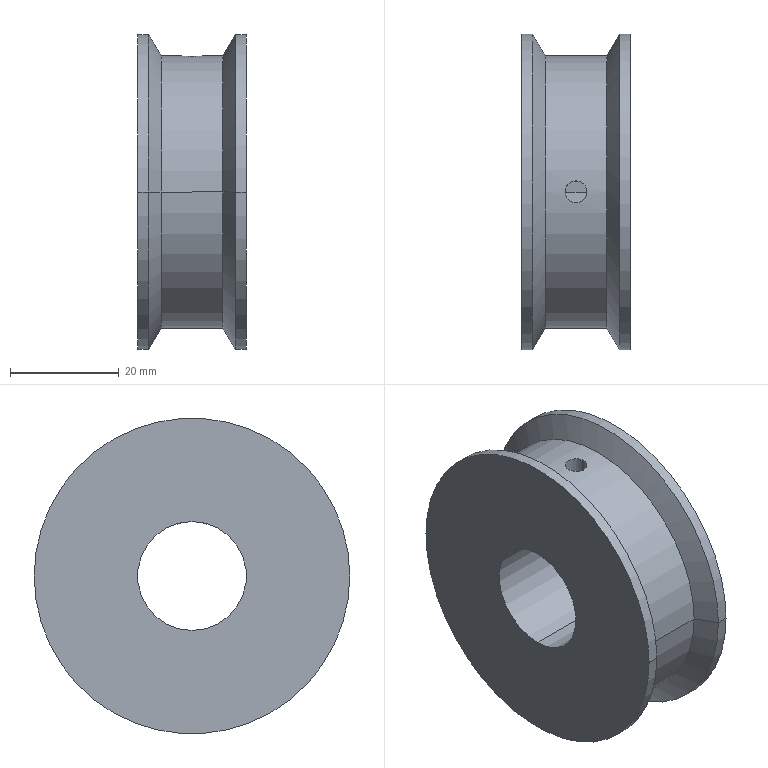Part | SolidWorks | features BaseBody 1 | 1 solid | 16 faces | box 20 x 58 x 58 mm | volume 37041 mm3 | cylinder 10 | cone 4 | plane 2 | commonest cylinder face diameters 58 x4 4 x2 20 x2 50 x2
STEP:
#1=CARTESIAN_POINT('',(2.,0.,10.));
#2=VERTEX_POINT('',#1);
#3=CARTESIAN_POINT('',(-2.,0.,10.));
#4=VERTEX_POINT('',#3);
#5=CARTESIAN_POINT('',(2.,0.,10.));
#6=CARTESIAN_POINT('',(2.,0.1325,10.));
#7=CARTESIAN_POINT('',(1.987,0.2627,9.997));
#8=CARTESIAN_POINT('',(1.936,0.5187,9.987));
#9=CARTESIAN_POINT('',(1.897,0.6459,9.98));
#10=CARTESIAN_POINT('',(1.797,0.8879,9.961));
#11=CARTESIAN_POINT('',(1.735,1.003,9.95));
#12=CARTESIAN_POINT('',(1.59,1.22,9.926));
#13=CARTESIAN_POINT('',(1.506,1.322,9.913));
#14=CARTESIAN_POINT('',(1.23,1.598,9.873));
#15=CARTESIAN_POINT('',(1.008,1.747,9.847));
#16=CARTESIAN_POINT('',(0.5268,1.947,9.809));
#17=CARTESIAN_POINT('',(0.2632,2.,9.798));
#18=CARTESIAN_POINT('',(-0.1291,2.,9.798));
#19=CARTESIAN_POINT('',(-0.262,1.987,9.801));
#20=CARTESIAN_POINT('',(-0.5188,1.936,9.811));
#21=CARTESIAN_POINT('',(-0.6436,1.898,9.818));
#22=CARTESIAN_POINT('',(-1.007,1.748,9.847));
#23=CARTESIAN_POINT('',(-1.227,1.601,9.873));
#24=CARTESIAN_POINT('',(-1.506,1.322,9.913));
#25=CARTESIAN_POINT('',(-1.589,1.222,9.926));
#26=CARTESIAN_POINT('',(-1.734,1.005,9.95));
#27=CARTESIAN_POINT('',(-1.797,0.8883,9.961));
#28=CARTESIAN_POINT('',(-1.897,0.6467,9.98));
#29=CARTESIAN_POINT('',(-1.935,0.522,9.987));
#30=CARTESIAN_POINT('',(-1.987,0.2651,9.997));
#31=CARTESIAN_POINT('',(-2.,0.1325,10.));
#32=CARTESIAN_POINT('',(-2.,0.,10.));
#33=B_SPLINE_CURVE_WITH_KNOTS('',3,(#5,#6,#7,#8,#9,#10,#11,#12,#13,#14,#15,#16,#17,#18,#19,#20,#21,#22,#23,#24,#25,#26,#27,#28,#29,#30,#31,#32),.UNSPECIFIED.,.F.,.F.,(4,2,2,2,2,2,2,2,2,2,2,2,2,4),(0.,0.0003917,0.0007834,0.001175,0.001567,0.00235,0.003134,0.003525,0.003917,0.0047,0.005092,0.005484,0.005875,0.006267),.UNSPECIFIED.);
#34=EDGE_CURVE('',#2,#4,#33,.T.);
#35=ORIENTED_EDGE('',*,*,#34,.F.);
#36=CARTESIAN_POINT('',(2.,0.,25.));
#37=VERTEX_POINT('',#36);
#38=CARTESIAN_POINT('',(2.,0.,25.));
#39=DIRECTION('',(0.,0.,1.));
#40=VECTOR('',#39,1000.);
#41=LINE('',#38,#40);
#42=EDGE_CURVE('',#2,#37,#41,.T.);
#43=ORIENTED_EDGE('',*,*,#42,.T.);
#44=CARTESIAN_POINT('',(-2.,0.,25.));
#45=VERTEX_POINT('',#44);
#46=CARTESIAN_POINT('',(-2.,0.,25.));
#47=CARTESIAN_POINT('',(-2.,0.1322,25.));
#48=CARTESIAN_POINT('',(-1.987,0.2621,24.999));
#49=CARTESIAN_POINT('',(-1.936,0.5178,24.995));
#50=CARTESIAN_POINT('',(-1.898,0.6448,24.992));
#51=CARTESIAN_POINT('',(-1.797,0.887,24.985));
#52=CARTESIAN_POINT('',(-1.736,1.002,24.98));
#53=CARTESIAN_POINT('',(-1.591,1.219,24.97));
#54=CARTESIAN_POINT('',(-1.506,1.322,24.965));
#55=CARTESIAN_POINT('',(-1.23,1.599,24.95));
#56=CARTESIAN_POINT('',(-1.007,1.748,24.939));
#57=CARTESIAN_POINT('',(-0.5256,1.947,24.924));
#58=CARTESIAN_POINT('',(-0.2623,2.,24.92));
#59=CARTESIAN_POINT('',(0.1291,2.,24.92));
#60=CARTESIAN_POINT('',(0.2616,1.987,24.921));
#61=CARTESIAN_POINT('',(0.5181,1.936,24.925));
#62=CARTESIAN_POINT('',(0.6428,1.898,24.928));
#63=CARTESIAN_POINT('',(0.885,1.798,24.935));
#64=CARTESIAN_POINT('',(1.002,1.736,24.94));
#65=CARTESIAN_POINT('',(1.219,1.591,24.949));
#66=CARTESIAN_POINT('',(1.32,1.508,24.955));
#67=CARTESIAN_POINT('',(1.507,1.322,24.965));
#68=CARTESIAN_POINT('',(1.589,1.221,24.97));
#69=CARTESIAN_POINT('',(1.734,1.004,24.98));
#70=CARTESIAN_POINT('',(1.797,0.8876,24.985));
#71=CARTESIAN_POINT('',(1.898,0.6454,24.992));
#72=CARTESIAN_POINT('',(1.935,0.5207,24.995));
#73=CARTESIAN_POINT('',(1.987,0.2645,24.999));
#74=CARTESIAN_POINT('',(2.,0.1322,25.));
#75=CARTESIAN_POINT('',(2.,0.,25.));
#76=B_SPLINE_CURVE_WITH_KNOTS('',3,(#46,#47,#48,#49,#50,#51,#52,#53,#54,#55,#56,#57,#58,#59,#60,#61,#62,#63,#64,#65,#66,#67,#68,#69,#70,#71,#72,#73,#74,#75),.UNSPECIFIED.,.F.,.F.,(4,2,2,2,2,2,2,2,2,2,2,2,2,2,4),(0.,0.0003909,0.0007818,0.001173,0.001564,0.002345,0.003127,0.003518,0.003909,0.0043,0.004691,0.005081,0.005472,0.005863,0.006254),.UNSPECIFIED.);
#77=EDGE_CURVE('',#45,#37,#76,.T.);
#78=ORIENTED_EDGE('',*,*,#77,.F.);
#79=CARTESIAN_POINT('',(-2.,0.,25.));
#80=DIRECTION('',(0.,0.,1.));
#81=VECTOR('',#80,1000.);
#82=LINE('',#79,#81);
#83=EDGE_CURVE('',#4,#45,#82,.T.);
#84=ORIENTED_EDGE('',*,*,#83,.F.);
#85=EDGE_LOOP('',(#35,#43,#78,#84));
#86=FACE_OUTER_BOUND('',#85,.T.);
#87=CARTESIAN_POINT('',(0.,0.,25.));
#88=DIRECTION('',(0.,0.,1.));
#89=DIRECTION('',(-1.,0.,0.));
#90=AXIS2_PLACEMENT_3D('',#87,#88,#89);
#91=CYLINDRICAL_SURFACE('',#90,2.);
#92=ADVANCED_FACE('',(#86),#91,.F.);
#93=CARTESIAN_POINT('',(-10.,0.,-10.));
#94=VERTEX_POINT('',#93);
#95=CARTESIAN_POINT('',(-10.,0.,10.));
#96=VERTEX_POINT('',#95);
#97=CARTESIAN_POINT('',(-10.,0.,0.));
#98=DIRECTION('',(1.,0.,0.));
#99=DIRECTION('',(0.,0.,1.));
#100=AXIS2_PLACEMENT_3D('',#97,#98,#99);
#101=CIRCLE('',#100,10.);
#102=EDGE_CURVE('',#94,#96,#101,.T.);
#103=ORIENTED_EDGE('',*,*,#102,.F.);
#104=CARTESIAN_POINT('',(10.,0.,-10.));
#105=VERTEX_POINT('',#104);
#106=CARTESIAN_POINT('',(10.,0.,-10.));
#107=DIRECTION('',(1.,0.,0.));
#108=VECTOR('',#107,1000.);
#109=LINE('',#106,#108);
#110=EDGE_CURVE('',#94,#105,#109,.T.);
#111=ORIENTED_EDGE('',*,*,#110,.T.);
#112=CARTESIAN_POINT('',(10.,0.,10.));
#113=VERTEX_POINT('',#112);
#114=CARTESIAN_POINT('',(10.,0.,0.));
#115=DIRECTION('',(-1.,0.,0.));
#116=DIRECTION('',(0.,0.,1.));
#117=AXIS2_PLACEMENT_3D('',#114,#115,#116);
#118=CIRCLE('',#117,10.);
#119=EDGE_CURVE('',#113,#105,#118,.T.);
#120=ORIENTED_EDGE('',*,*,#119,.F.);
#121=CARTESIAN_POINT('',(10.,0.,10.));
#122=DIRECTION('',(1.,0.,0.));
#123=VECTOR('',#122,1000.);
#124=LINE('',#121,#123);
#125=EDGE_CURVE('',#2,#113,#124,.T.);
#126=ORIENTED_EDGE('',*,*,#125,.F.);
#127=ORIENTED_EDGE('',*,*,#34,.T.);
#128=CARTESIAN_POINT('',(10.,0.,10.));
#129=DIRECTION('',(1.,0.,0.));
#130=VECTOR('',#129,1000.);
#131=LINE('',#128,#130);
#132=EDGE_CURVE('',#96,#4,#131,.T.);
#133=ORIENTED_EDGE('',*,*,#132,.F.);
#134=EDGE_LOOP('',(#103,#111,#120,#126,#127,#133));
#135=FACE_OUTER_BOUND('',#134,.T.);
#136=CARTESIAN_POINT('',(10.,0.,0.));
#137=DIRECTION('',(1.,0.,0.));
#138=DIRECTION('',(0.,0.,1.));
#139=AXIS2_PLACEMENT_3D('',#136,#137,#138);
#140=CYLINDRICAL_SURFACE('',#139,10.);
#141=ADVANCED_FACE('',(#135),#140,.F.);
#142=CARTESIAN_POINT('',(-8.,-29.,0.));
#143=VERTEX_POINT('',#142);
#144=CARTESIAN_POINT('',(-8.,29.,0.));
#145=VERTEX_POINT('',#144);
#146=CARTESIAN_POINT('',(-8.,0.,0.));
#147=DIRECTION('',(1.,0.,0.));
#148=DIRECTION('',(0.,0.,-1.));
#149=AXIS2_PLACEMENT_3D('',#146,#147,#148);
#150=CIRCLE('',#149,29.);
#151=EDGE_CURVE('',#143,#145,#150,.T.);
#152=ORIENTED_EDGE('',*,*,#151,.F.);
#153=CARTESIAN_POINT('',(-10.,-29.,0.));
#154=VERTEX_POINT('',#153);
#155=CARTESIAN_POINT('',(-9.,-29.,0.));
#156=DIRECTION('',(-1.,0.,0.));
#157=VECTOR('',#156,1000.);
#158=LINE('',#155,#157);
#159=EDGE_CURVE('',#143,#154,#158,.T.);
#160=ORIENTED_EDGE('',*,*,#159,.T.);
#161=CARTESIAN_POINT('',(-10.,29.,0.));
#162=VERTEX_POINT('',#161);
#163=CARTESIAN_POINT('',(-10.,0.,0.));
#164=DIRECTION('',(1.,0.,0.));
#165=DIRECTION('',(0.,0.,-1.));
#166=AXIS2_PLACEMENT_3D('',#163,#164,#165);
#167=CIRCLE('',#166,29.);
#168=EDGE_CURVE('',#154,#162,#167,.T.);
#169=ORIENTED_EDGE('',*,*,#168,.T.);
#170=CARTESIAN_POINT('',(-9.,29.,0.));
#171=DIRECTION('',(-1.,0.,0.));
#172=VECTOR('',#171,1000.);
#173=LINE('',#170,#172);
#174=EDGE_CURVE('',#145,#162,#173,.T.);
#175=ORIENTED_EDGE('',*,*,#174,.F.);
#176=EDGE_LOOP('',(#152,#160,#169,#175));
#177=FACE_OUTER_BOUND('',#176,.T.);
#178=CARTESIAN_POINT('',(-9.,0.,0.));
#179=DIRECTION('',(-1.,0.,0.));
#180=DIRECTION('',(0.,1.,0.));
#181=AXIS2_PLACEMENT_3D('',#178,#179,#180);
#182=CYLINDRICAL_SURFACE('',#181,29.);
#183=ADVANCED_FACE('',(#177),#182,.T.);
#184=CARTESIAN_POINT('',(-5.691,-25.,0.));
#185=VERTEX_POINT('',#184);
#186=CARTESIAN_POINT('',(-5.691,25.,0.));
#187=VERTEX_POINT('',#186);
#188=CARTESIAN_POINT('',(-5.691,0.,0.));
#189=DIRECTION('',(1.,0.,0.));
#190=DIRECTION('',(0.,0.,-1.));
#191=AXIS2_PLACEMENT_3D('',#188,#189,#190);
#192=CIRCLE('',#191,25.);
#193=EDGE_CURVE('',#185,#187,#192,.T.);
#194=ORIENTED_EDGE('',*,*,#193,.F.);
#195=CARTESIAN_POINT('',(-6.845,-27.,0.));
#196=DIRECTION('',(-0.5,-0.866,0.));
#197=VECTOR('',#196,1000.);
#198=LINE('',#195,#197);
#199=EDGE_CURVE('',#185,#143,#198,.T.);
#200=ORIENTED_EDGE('',*,*,#199,.T.);
#201=ORIENTED_EDGE('',*,*,#151,.T.);
#202=CARTESIAN_POINT('',(-6.845,27.,0.));
#203=DIRECTION('',(-0.5,0.866,0.));
#204=VECTOR('',#203,1000.);
#205=LINE('',#202,#204);
#206=EDGE_CURVE('',#187,#145,#205,.T.);
#207=ORIENTED_EDGE('',*,*,#206,.F.);
#208=EDGE_LOOP('',(#194,#200,#201,#207));
#209=FACE_OUTER_BOUND('',#208,.T.);
#210=CARTESIAN_POINT('',(-6.845,0.,0.));
#211=DIRECTION('',(-1.,0.,0.));
#212=DIRECTION('',(0.,1.,0.));
#213=AXIS2_PLACEMENT_3D('',#210,#211,#212);
#214=CONICAL_SURFACE('',#213,27.,1.047);
#215=ADVANCED_FACE('',(#209),#214,.T.);
#216=CARTESIAN_POINT('',(5.691,-25.,0.));
#217=VERTEX_POINT('',#216);
#218=CARTESIAN_POINT('',(5.691,25.,0.));
#219=VERTEX_POINT('',#218);
#220=CARTESIAN_POINT('',(5.691,0.,0.));
#221=DIRECTION('',(1.,0.,0.));
#222=DIRECTION('',(0.,0.,-1.));
#223=AXIS2_PLACEMENT_3D('',#220,#221,#222);
#224=CIRCLE('',#223,25.);
#225=EDGE_CURVE('',#217,#219,#224,.T.);
#226=ORIENTED_EDGE('',*,*,#225,.F.);
#227=CARTESIAN_POINT('',(0.,-25.,0.));
#228=DIRECTION('',(-1.,0.,0.));
#229=VECTOR('',#228,1000.);
#230=LINE('',#227,#229);
#231=EDGE_CURVE('',#217,#185,#230,.T.);
#232=ORIENTED_EDGE('',*,*,#231,.T.);
#233=ORIENTED_EDGE('',*,*,#193,.T.);
#234=CARTESIAN_POINT('',(0.,25.,0.));
#235=DIRECTION('',(-1.,0.,0.));
#236=VECTOR('',#235,1000.);
#237=LINE('',#234,#236);
#238=EDGE_CURVE('',#219,#187,#237,.T.);
#239=ORIENTED_EDGE('',*,*,#238,.F.);
#240=EDGE_LOOP('',(#226,#232,#233,#239));
#241=FACE_OUTER_BOUND('',#240,.T.);
#242=CARTESIAN_POINT('',(0.,0.,0.));
#243=DIRECTION('',(-1.,0.,0.));
#244=DIRECTION('',(0.,1.,0.));
#245=AXIS2_PLACEMENT_3D('',#242,#243,#244);
#246=CYLINDRICAL_SURFACE('',#245,25.);
#247=ADVANCED_FACE('',(#241),#246,.T.);
#248=CARTESIAN_POINT('',(5.691,0.,0.));
#249=DIRECTION('',(1.,0.,0.));
#250=DIRECTION('',(0.,0.,-1.));
#251=AXIS2_PLACEMENT_3D('',#248,#249,#250);
#252=CIRCLE('',#251,25.);
#253=EDGE_CURVE('',#219,#217,#252,.T.);
#254=ORIENTED_EDGE('',*,*,#253,.T.);
#255=CARTESIAN_POINT('',(8.,-29.,0.));
#256=VERTEX_POINT('',#255);
#257=CARTESIAN_POINT('',(6.845,-27.,0.));
#258=DIRECTION('',(0.5,-0.866,0.));
#259=VECTOR('',#258,1000.);
#260=LINE('',#257,#259);
#261=EDGE_CURVE('',#217,#256,#260,.T.);
#262=ORIENTED_EDGE('',*,*,#261,.T.);
#263=CARTESIAN_POINT('',(8.,29.,0.));
#264=VERTEX_POINT('',#263);
#265=CARTESIAN_POINT('',(8.,0.,0.));
#266=DIRECTION('',(1.,0.,0.));
#267=DIRECTION('',(0.,0.,-1.));
#268=AXIS2_PLACEMENT_3D('',#265,#266,#267);
#269=CIRCLE('',#268,29.);
#270=EDGE_CURVE('',#264,#256,#269,.T.);
#271=ORIENTED_EDGE('',*,*,#270,.F.);
#272=CARTESIAN_POINT('',(6.845,27.,0.));
#273=DIRECTION('',(0.5,0.866,0.));
#274=VECTOR('',#273,1000.);
#275=LINE('',#272,#274);
#276=EDGE_CURVE('',#219,#264,#275,.T.);
#277=ORIENTED_EDGE('',*,*,#276,.F.);
#278=EDGE_LOOP('',(#254,#262,#271,#277));
#279=FACE_OUTER_BOUND('',#278,.T.);
#280=CARTESIAN_POINT('',(6.845,0.,0.));
#281=DIRECTION('',(1.,0.,0.));
#282=DIRECTION('',(0.,1.,0.));
#283=AXIS2_PLACEMENT_3D('',#280,#281,#282);
#284=CONICAL_SURFACE('',#283,27.,1.047);
#285=ADVANCED_FACE('',(#279),#284,.T.);
#286=CARTESIAN_POINT('',(10.,-29.,0.));
#287=VERTEX_POINT('',#286);
#288=CARTESIAN_POINT('',(10.,29.,0.));
#289=VERTEX_POINT('',#288);
#290=CARTESIAN_POINT('',(10.,0.,0.));
#291=DIRECTION('',(1.,0.,0.));
#292=DIRECTION('',(0.,0.,-1.));
#293=AXIS2_PLACEMENT_3D('',#290,#291,#292);
#294=CIRCLE('',#293,29.);
#295=EDGE_CURVE('',#287,#289,#294,.T.);
#296=ORIENTED_EDGE('',*,*,#295,.F.);
#297=CARTESIAN_POINT('',(9.,-29.,0.));
#298=DIRECTION('',(-1.,0.,0.));
#299=VECTOR('',#298,1000.);
#300=LINE('',#297,#299);
#301=EDGE_CURVE('',#287,#256,#300,.T.);
#302=ORIENTED_EDGE('',*,*,#301,.T.);
#303=CARTESIAN_POINT('',(8.,0.,0.));
#304=DIRECTION('',(1.,0.,0.));
#305=DIRECTION('',(0.,0.,-1.));
#306=AXIS2_PLACEMENT_3D('',#303,#304,#305);
#307=CIRCLE('',#306,29.);
#308=EDGE_CURVE('',#256,#264,#307,.T.);
#309=ORIENTED_EDGE('',*,*,#308,.T.);
#310=CARTESIAN_POINT('',(9.,29.,0.));
#311=DIRECTION('',(-1.,0.,0.));
#312=VECTOR('',#311,1000.);
#313=LINE('',#310,#312);
#314=EDGE_CURVE('',#289,#264,#313,.T.);
#315=ORIENTED_EDGE('',*,*,#314,.F.);
#316=EDGE_LOOP('',(#296,#302,#309,#315));
#317=FACE_OUTER_BOUND('',#316,.T.);
#318=CARTESIAN_POINT('',(9.,0.,0.));
#319=DIRECTION('',(-1.,0.,0.));
#320=DIRECTION('',(0.,1.,0.));
#321=AXIS2_PLACEMENT_3D('',#318,#319,#320);
#322=CYLINDRICAL_SURFACE('',#321,29.);
#323=ADVANCED_FACE('',(#317),#322,.T.);
#324=CARTESIAN_POINT('',(-10.,0.,0.));
#325=DIRECTION('',(1.,0.,0.));
#326=DIRECTION('',(0.,0.,1.));
#327=AXIS2_PLACEMENT_3D('',#324,#325,#326);
#328=CIRCLE('',#327,10.);
#329=EDGE_CURVE('',#96,#94,#328,.T.);
#330=ORIENTED_EDGE('',*,*,#329,.T.);
#331=ORIENTED_EDGE('',*,*,#102,.T.);
#332=EDGE_LOOP('',(#330,#331));
#333=FACE_BOUND('',#332,.T.);
#334=CARTESIAN_POINT('',(-10.,0.,0.));
#335=DIRECTION('',(1.,0.,0.));
#336=DIRECTION('',(0.,0.,-1.));
#337=AXIS2_PLACEMENT_3D('',#334,#335,#336);
#338=CIRCLE('',#337,29.);
#339=EDGE_CURVE('',#162,#154,#338,.T.);
#340=ORIENTED_EDGE('',*,*,#339,.F.);
#341=ORIENTED_EDGE('',*,*,#168,.F.);
#342=EDGE_LOOP('',(#340,#341));
#343=FACE_OUTER_BOUND('',#342,.T.);
#344=CARTESIAN_POINT('',(-10.,29.,0.));
#345=DIRECTION('',(-1.,0.,0.));
#346=DIRECTION('',(0.,0.,1.));
#347=AXIS2_PLACEMENT_3D('',#344,#345,#346);
#348=PLANE('',#347);
#349=ADVANCED_FACE('',(#333,#343),#348,.T.);
#350=ORIENTED_EDGE('',*,*,#119,.T.);
#351=CARTESIAN_POINT('',(10.,0.,0.));
#352=DIRECTION('',(-1.,0.,0.));
#353=DIRECTION('',(0.,0.,1.));
#354=AXIS2_PLACEMENT_3D('',#351,#352,#353);
#355=CIRCLE('',#354,10.);
#356=EDGE_CURVE('',#105,#113,#355,.T.);
#357=ORIENTED_EDGE('',*,*,#356,.T.);
#358=EDGE_LOOP('',(#350,#357));
#359=FACE_BOUND('',#358,.T.);
#360=CARTESIAN_POINT('',(10.,0.,0.));
#361=DIRECTION('',(1.,0.,0.));
#362=DIRECTION('',(0.,0.,-1.));
#363=AXIS2_PLACEMENT_3D('',#360,#361,#362);
#364=CIRCLE('',#363,29.);
#365=EDGE_CURVE('',#289,#287,#364,.T.);
#366=ORIENTED_EDGE('',*,*,#365,.T.);
#367=ORIENTED_EDGE('',*,*,#295,.T.);
#368=EDGE_LOOP('',(#366,#367));
#369=FACE_OUTER_BOUND('',#368,.T.);
#370=CARTESIAN_POINT('',(10.,0.,0.));
#371=DIRECTION('',(1.,0.,0.));
#372=DIRECTION('',(0.,1.,0.));
#373=AXIS2_PLACEMENT_3D('',#370,#371,#372);
#374=PLANE('',#373);
#375=ADVANCED_FACE('',(#359,#369),#374,.T.);
#376=ORIENTED_EDGE('',*,*,#301,.F.);
#377=ORIENTED_EDGE('',*,*,#365,.F.);
#378=ORIENTED_EDGE('',*,*,#314,.T.);
#379=ORIENTED_EDGE('',*,*,#270,.T.);
#380=EDGE_LOOP('',(#376,#377,#378,#379));
#381=FACE_OUTER_BOUND('',#380,.T.);
#382=CARTESIAN_POINT('',(9.,0.,0.));
#383=DIRECTION('',(-1.,0.,0.));
#384=DIRECTION('',(0.,1.,0.));
#385=AXIS2_PLACEMENT_3D('',#382,#383,#384);
#386=CYLINDRICAL_SURFACE('',#385,29.);
#387=ADVANCED_FACE('',(#381),#386,.T.);
#388=ORIENTED_EDGE('',*,*,#261,.F.);
#389=ORIENTED_EDGE('',*,*,#225,.T.);
#390=ORIENTED_EDGE('',*,*,#276,.T.);
#391=ORIENTED_EDGE('',*,*,#308,.F.);
#392=EDGE_LOOP('',(#388,#389,#390,#391));
#393=FACE_OUTER_BOUND('',#392,.T.);
#394=CARTESIAN_POINT('',(6.845,0.,0.));
#395=DIRECTION('',(1.,0.,0.));
#396=DIRECTION('',(0.,1.,0.));
#397=AXIS2_PLACEMENT_3D('',#394,#395,#396);
#398=CONICAL_SURFACE('',#397,27.,1.047);
#399=ADVANCED_FACE('',(#393),#398,.T.);
#400=ORIENTED_EDGE('',*,*,#231,.F.);
#401=ORIENTED_EDGE('',*,*,#253,.F.);
#402=ORIENTED_EDGE('',*,*,#238,.T.);
#403=CARTESIAN_POINT('',(-5.691,0.,0.));
#404=DIRECTION('',(1.,0.,0.));
#405=DIRECTION('',(0.,0.,-1.));
#406=AXIS2_PLACEMENT_3D('',#403,#404,#405);
#407=CIRCLE('',#406,25.);
#408=EDGE_CURVE('',#187,#185,#407,.T.);
#409=ORIENTED_EDGE('',*,*,#408,.T.);
#410=EDGE_LOOP('',(#400,#401,#402,#409));
#411=FACE_OUTER_BOUND('',#410,.T.);
#412=ORIENTED_EDGE('',*,*,#77,.T.);
#413=CARTESIAN_POINT('',(2.,0.,25.));
#414=CARTESIAN_POINT('',(2.,-0.1322,25.));
#415=CARTESIAN_POINT('',(1.987,-0.2621,24.999));
#416=CARTESIAN_POINT('',(1.936,-0.5178,24.995));
#417=CARTESIAN_POINT('',(1.898,-0.6448,24.992));
#418=CARTESIAN_POINT('',(1.797,-0.887,24.985));
#419=CARTESIAN_POINT('',(1.736,-1.002,24.98));
#420=CARTESIAN_POINT('',(1.591,-1.219,24.97));
#421=CARTESIAN_POINT('',(1.506,-1.322,24.965));
#422=CARTESIAN_POINT('',(1.23,-1.599,24.95));
#423=CARTESIAN_POINT('',(1.007,-1.748,24.939));
#424=CARTESIAN_POINT('',(0.5256,-1.947,24.924));
#425=CARTESIAN_POINT('',(0.2623,-2.,24.92));
#426=CARTESIAN_POINT('',(-0.1291,-2.,24.92));
#427=CARTESIAN_POINT('',(-0.2616,-1.987,24.921));
#428=CARTESIAN_POINT('',(-0.5181,-1.936,24.925));
#429=CARTESIAN_POINT('',(-0.6428,-1.898,24.928));
#430=CARTESIAN_POINT('',(-0.885,-1.798,24.935));
#431=CARTESIAN_POINT('',(-1.002,-1.736,24.94));
#432=CARTESIAN_POINT('',(-1.219,-1.591,24.949));
#433=CARTESIAN_POINT('',(-1.32,-1.508,24.955));
#434=CARTESIAN_POINT('',(-1.507,-1.322,24.965));
#435=CARTESIAN_POINT('',(-1.589,-1.221,24.97));
#436=CARTESIAN_POINT('',(-1.734,-1.004,24.98));
#437=CARTESIAN_POINT('',(-1.797,-0.8876,24.985));
#438=CARTESIAN_POINT('',(-1.898,-0.6454,24.992));
#439=CARTESIAN_POINT('',(-1.935,-0.5207,24.995));
#440=CARTESIAN_POINT('',(-1.987,-0.2645,24.999));
#441=CARTESIAN_POINT('',(-2.,-0.1322,25.));
#442=CARTESIAN_POINT('',(-2.,0.,25.));
#443=B_SPLINE_CURVE_WITH_KNOTS('',3,(#413,#414,#415,#416,#417,#418,#419,#420,#421,#422,#423,#424,#425,#426,#427,#428,#429,#430,#431,#432,#433,#434,#435,#436,#437,#438,#439,#440,#441,#442),.UNSPECIFIED.,.F.,.F.,(4,2,2,2,2,2,2,2,2,2,2,2,2,2,4),(0.006254,0.006645,0.007036,0.007427,0.007818,0.008599,0.009381,0.009772,0.01016,0.01055,0.01094,0.01134,0.01173,0.01212,0.01251),.UNSPECIFIED.);
#444=EDGE_CURVE('',#37,#45,#443,.T.);
#445=ORIENTED_EDGE('',*,*,#444,.T.);
#446=EDGE_LOOP('',(#412,#445));
#447=FACE_BOUND('',#446,.T.);
#448=CARTESIAN_POINT('',(0.,0.,0.));
#449=DIRECTION('',(-1.,0.,0.));
#450=DIRECTION('',(0.,1.,0.));
#451=AXIS2_PLACEMENT_3D('',#448,#449,#450);
#452=CYLINDRICAL_SURFACE('',#451,25.);
#453=ADVANCED_FACE('',(#411,#447),#452,.T.);
#454=ORIENTED_EDGE('',*,*,#199,.F.);
#455=ORIENTED_EDGE('',*,*,#408,.F.);
#456=ORIENTED_EDGE('',*,*,#206,.T.);
#457=CARTESIAN_POINT('',(-8.,0.,0.));
#458=DIRECTION('',(1.,0.,0.));
#459=DIRECTION('',(0.,0.,-1.));
#460=AXIS2_PLACEMENT_3D('',#457,#458,#459);
#461=CIRCLE('',#460,29.);
#462=EDGE_CURVE('',#145,#143,#461,.T.);
#463=ORIENTED_EDGE('',*,*,#462,.T.);
#464=EDGE_LOOP('',(#454,#455,#456,#463));
#465=FACE_OUTER_BOUND('',#464,.T.);
#466=CARTESIAN_POINT('',(-6.845,0.,0.));
#467=DIRECTION('',(-1.,0.,0.));
#468=DIRECTION('',(0.,1.,0.));
#469=AXIS2_PLACEMENT_3D('',#466,#467,#468);
#470=CONICAL_SURFACE('',#469,27.,1.047);
#471=ADVANCED_FACE('',(#465),#470,.T.);
#472=ORIENTED_EDGE('',*,*,#159,.F.);
#473=ORIENTED_EDGE('',*,*,#462,.F.);
#474=ORIENTED_EDGE('',*,*,#174,.T.);
#475=ORIENTED_EDGE('',*,*,#339,.T.);
#476=EDGE_LOOP('',(#472,#473,#474,#475));
#477=FACE_OUTER_BOUND('',#476,.T.);
#478=CARTESIAN_POINT('',(-9.,0.,0.));
#479=DIRECTION('',(-1.,0.,0.));
#480=DIRECTION('',(0.,1.,0.));
#481=AXIS2_PLACEMENT_3D('',#478,#479,#480);
#482=CYLINDRICAL_SURFACE('',#481,29.);
#483=ADVANCED_FACE('',(#477),#482,.T.);
#484=ORIENTED_EDGE('',*,*,#110,.F.);
#485=ORIENTED_EDGE('',*,*,#329,.F.);
#486=ORIENTED_EDGE('',*,*,#132,.T.);
#487=CARTESIAN_POINT('',(-2.,0.,10.));
#488=CARTESIAN_POINT('',(-2.,-0.1325,10.));
#489=CARTESIAN_POINT('',(-1.987,-0.2627,9.997));
#490=CARTESIAN_POINT('',(-1.936,-0.5187,9.987));
#491=CARTESIAN_POINT('',(-1.897,-0.6459,9.98));
#492=CARTESIAN_POINT('',(-1.797,-0.8879,9.961));
#493=CARTESIAN_POINT('',(-1.735,-1.003,9.95));
#494=CARTESIAN_POINT('',(-1.59,-1.22,9.926));
#495=CARTESIAN_POINT('',(-1.506,-1.322,9.913));
#496=CARTESIAN_POINT('',(-1.23,-1.598,9.873));
#497=CARTESIAN_POINT('',(-1.008,-1.747,9.847));
#498=CARTESIAN_POINT('',(-0.5268,-1.947,9.809));
#499=CARTESIAN_POINT('',(-0.2632,-2.,9.798));
#500=CARTESIAN_POINT('',(0.1291,-2.,9.798));
#501=CARTESIAN_POINT('',(0.262,-1.987,9.801));
#502=CARTESIAN_POINT('',(0.5188,-1.936,9.811));
#503=CARTESIAN_POINT('',(0.6436,-1.898,9.818));
#504=CARTESIAN_POINT('',(1.007,-1.748,9.847));
#505=CARTESIAN_POINT('',(1.227,-1.601,9.873));
#506=CARTESIAN_POINT('',(1.506,-1.322,9.913));
#507=CARTESIAN_POINT('',(1.589,-1.222,9.926));
#508=CARTESIAN_POINT('',(1.734,-1.005,9.95));
#509=CARTESIAN_POINT('',(1.797,-0.8883,9.961));
#510=CARTESIAN_POINT('',(1.897,-0.6467,9.98));
#511=CARTESIAN_POINT('',(1.935,-0.522,9.987));
#512=CARTESIAN_POINT('',(1.987,-0.2651,9.997));
#513=CARTESIAN_POINT('',(2.,-0.1325,10.));
#514=CARTESIAN_POINT('',(2.,0.,10.));
#515=B_SPLINE_CURVE_WITH_KNOTS('',3,(#487,#488,#489,#490,#491,#492,#493,#494,#495,#496,#497,#498,#499,#500,#501,#502,#503,#504,#505,#506,#507,#508,#509,#510,#511,#512,#513,#514),.UNSPECIFIED.,.F.,.F.,(4,2,2,2,2,2,2,2,2,2,2,2,2,4),(0.006267,0.006659,0.00705,0.007442,0.007834,0.008617,0.009401,0.009792,0.01018,0.01097,0.01136,0.01175,0.01214,0.01253),.UNSPECIFIED.);
#516=EDGE_CURVE('',#4,#2,#515,.T.);
#517=ORIENTED_EDGE('',*,*,#516,.T.);
#518=ORIENTED_EDGE('',*,*,#125,.T.);
#519=ORIENTED_EDGE('',*,*,#356,.F.);
#520=EDGE_LOOP('',(#484,#485,#486,#517,#518,#519));
#521=FACE_OUTER_BOUND('',#520,.T.);
#522=CARTESIAN_POINT('',(10.,0.,0.));
#523=DIRECTION('',(1.,0.,0.));
#524=DIRECTION('',(0.,0.,1.));
#525=AXIS2_PLACEMENT_3D('',#522,#523,#524);
#526=CYLINDRICAL_SURFACE('',#525,10.);
#527=ADVANCED_FACE('',(#521),#526,.F.);
#528=ORIENTED_EDGE('',*,*,#42,.F.);
#529=ORIENTED_EDGE('',*,*,#516,.F.);
#530=ORIENTED_EDGE('',*,*,#83,.T.);
#531=ORIENTED_EDGE('',*,*,#444,.F.);
#532=EDGE_LOOP('',(#528,#529,#530,#531));
#533=FACE_OUTER_BOUND('',#532,.T.);
#534=CARTESIAN_POINT('',(0.,0.,25.));
#535=DIRECTION('',(0.,0.,1.));
#536=DIRECTION('',(-1.,0.,0.));
#537=AXIS2_PLACEMENT_3D('',#534,#535,#536);
#538=CYLINDRICAL_SURFACE('',#537,2.);
#539=ADVANCED_FACE('',(#533),#538,.F.);
#540=CLOSED_SHELL('',(#92,#141,#183,#215,#247,#285,#323,#349,#375,#387,#399,#453,#471,#483,#527,#539));
#541=MANIFOLD_SOLID_BREP('',#540);
#542=CARTESIAN_POINT('',(0.,0.,0.));
#543=DIRECTION('',(0.,0.,1.));
#544=DIRECTION('',(1.,0.,0.));
#545=AXIS2_PLACEMENT_3D('',#542,#543,#544);
#546=(LENGTH_UNIT()NAMED_UNIT(*)SI_UNIT(.MILLI.,.METRE.));
#547=UNCERTAINTY_MEASURE_WITH_UNIT(LENGTH_MEASURE(0.00001),#546,'','');
#548=(NAMED_UNIT(*)PLANE_ANGLE_UNIT()SI_UNIT($,.RADIAN.));
#549=(NAMED_UNIT(*)SI_UNIT($,.STERADIAN.)SOLID_ANGLE_UNIT());
#550=(GEOMETRIC_REPRESENTATION_CONTEXT(3)GLOBAL_UNCERTAINTY_ASSIGNED_CONTEXT((#547))GLOBAL_UNIT_ASSIGNED_CONTEXT((#546,#548,#549))REPRESENTATION_CONTEXT('',''));
#551=ADVANCED_BREP_SHAPE_REPRESENTATION('',(#541,#545),#550);